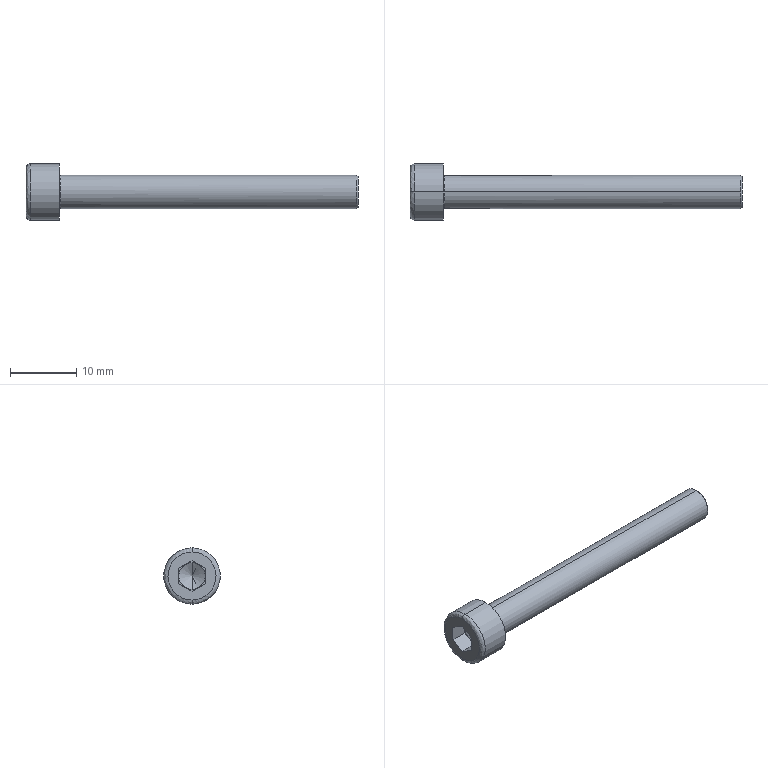Part | SolidWorks | features BaseBody 1 | 1 solid | 27 faces | box 50 x 8.5 x 8.5 mm | volume 1125 mm3 | plane 15 | spline 4 | cylinder 4 | cone 4 | commonest cylinder face diameters 5 x2 8.5 x2
STEP:
#1=CARTESIAN_POINT('',(5.,0.,2.7));
#2=VERTEX_POINT('',#1);
#3=CARTESIAN_POINT('',(5.,0.,-2.7));
#4=VERTEX_POINT('',#3);
#5=CARTESIAN_POINT('',(5.,0.,2.7));
#6=CARTESIAN_POINT('',(5.,0.1716,2.7));
#7=CARTESIAN_POINT('',(5.,0.4245,2.676));
#8=CARTESIAN_POINT('',(5.,0.7118,2.607));
#9=CARTESIAN_POINT('',(5.,0.8535,2.562));
#10=CARTESIAN_POINT('',(5.,0.9138,2.541));
#11=CARTESIAN_POINT('',(5.,0.9539,2.526));
#12=CARTESIAN_POINT('',(5.,0.9722,2.519));
#13=CARTESIAN_POINT('',(5.,1.34,2.373));
#14=CARTESIAN_POINT('',(5.,1.646,2.172));
#15=CARTESIAN_POINT('',(5.,2.041,1.778));
#16=CARTESIAN_POINT('',(5.,2.215,1.564));
#17=CARTESIAN_POINT('',(5.,2.376,1.288));
#18=CARTESIAN_POINT('',(5.,2.447,1.143));
#19=CARTESIAN_POINT('',(5.,2.475,1.08));
#20=CARTESIAN_POINT('',(5.,2.493,1.037));
#21=CARTESIAN_POINT('',(5.,2.503,1.014));
#22=CARTESIAN_POINT('',(5.,2.637,0.675));
#23=CARTESIAN_POINT('',(5.,2.7,0.343));
#24=CARTESIAN_POINT('',(5.,2.7,-0.1715));
#25=CARTESIAN_POINT('',(5.,2.676,-0.4243));
#26=CARTESIAN_POINT('',(5.,2.607,-0.7117));
#27=CARTESIAN_POINT('',(5.,2.562,-0.8534));
#28=CARTESIAN_POINT('',(5.,2.541,-0.9137));
#29=CARTESIAN_POINT('',(5.,2.526,-0.9539));
#30=CARTESIAN_POINT('',(5.,2.519,-0.9722));
#31=CARTESIAN_POINT('',(5.,2.373,-1.34));
#32=CARTESIAN_POINT('',(5.,2.172,-1.646));
#33=CARTESIAN_POINT('',(5.,1.778,-2.041));
#34=CARTESIAN_POINT('',(5.,1.564,-2.215));
#35=CARTESIAN_POINT('',(5.,1.288,-2.376));
#36=CARTESIAN_POINT('',(5.,1.143,-2.447));
#37=CARTESIAN_POINT('',(5.,1.08,-2.475));
#38=CARTESIAN_POINT('',(5.,1.037,-2.493));
#39=CARTESIAN_POINT('',(5.,1.014,-2.503));
#40=CARTESIAN_POINT('',(5.,0.6748,-2.637));
#41=CARTESIAN_POINT('',(5.,0.3435,-2.7));
#42=CARTESIAN_POINT('',(5.,0.,-2.7));
#43=B_SPLINE_CURVE_WITH_KNOTS('',3,(#5,#6,#7,#8,#9,#10,#11,#12,#13,#14,#15,#16,#17,#18,#19,#20,#21,#22,#23,#24,#25,#26,#27,#28,#29,#30,#31,#32,#33,#34,#35,#36,#37,#38,#39,#40,#41,#42),.UNSPECIFIED.,.F.,.F.,(4,1,1,1,2,2,2,1,1,1,2,2,2,1,1,1,2,2,2,1,1,1,2,2,4),(0.,0.0625,0.09375,0.1094,0.1172,0.125,0.25,0.3125,0.3437,0.3594,0.3672,0.375,0.5,0.5625,0.5937,0.6094,0.6172,0.625,0.75,0.8125,0.8437,0.8594,0.8672,0.875,1.),.UNSPECIFIED.);
#44=EDGE_CURVE('',#2,#4,#43,.T.);
#45=ORIENTED_EDGE('',*,*,#44,.F.);
#46=CARTESIAN_POINT('',(5.2,0.,2.5));
#47=VERTEX_POINT('',#46);
#48=CARTESIAN_POINT('',(5.2,0.,2.7));
#49=DIRECTION('',(0.,-1.,0.));
#50=DIRECTION('',(0.,0.,1.));
#51=AXIS2_PLACEMENT_3D('',#48,#49,#50);
#52=CIRCLE('',#51,0.2);
#53=EDGE_CURVE('',#2,#47,#52,.T.);
#54=ORIENTED_EDGE('',*,*,#53,.T.);
#55=CARTESIAN_POINT('',(5.2,0.,-2.5));
#56=VERTEX_POINT('',#55);
#57=CARTESIAN_POINT('',(5.2,0.,0.));
#58=DIRECTION('',(1.,0.,0.));
#59=DIRECTION('',(0.,0.,1.));
#60=AXIS2_PLACEMENT_3D('',#57,#58,#59);
#61=CIRCLE('',#60,2.5);
#62=EDGE_CURVE('',#56,#47,#61,.T.);
#63=ORIENTED_EDGE('',*,*,#62,.F.);
#64=CARTESIAN_POINT('',(5.2,0.,-2.7));
#65=DIRECTION('',(0.,1.,0.));
#66=DIRECTION('',(0.,0.,-1.));
#67=AXIS2_PLACEMENT_3D('',#64,#65,#66);
#68=CIRCLE('',#67,0.2);
#69=EDGE_CURVE('',#4,#56,#68,.T.);
#70=ORIENTED_EDGE('',*,*,#69,.F.);
#71=EDGE_LOOP('',(#45,#54,#63,#70));
#72=FACE_OUTER_BOUND('',#71,.T.);
#73=CARTESIAN_POINT('',(5.,0.,-2.7));
#74=CARTESIAN_POINT('',(5.,5.4,-2.7));
#75=CARTESIAN_POINT('',(5.,5.4,2.7));
#76=CARTESIAN_POINT('',(5.,0.,2.7));
#77=CARTESIAN_POINT('',(5.,0.,-2.583));
#78=CARTESIAN_POINT('',(5.,5.166,-2.583));
#79=CARTESIAN_POINT('',(5.,5.166,2.583));
#80=CARTESIAN_POINT('',(5.,0.,2.583));
#81=CARTESIAN_POINT('',(5.083,0.,-2.5));
#82=CARTESIAN_POINT('',(5.083,5.,-2.5));
#83=CARTESIAN_POINT('',(5.083,5.,2.5));
#84=CARTESIAN_POINT('',(5.083,0.,2.5));
#85=CARTESIAN_POINT('',(5.2,0.,-2.5));
#86=CARTESIAN_POINT('',(5.2,5.,-2.5));
#87=CARTESIAN_POINT('',(5.2,5.,2.5));
#88=CARTESIAN_POINT('',(5.2,0.,2.5));
#89=(BOUNDED_SURFACE()B_SPLINE_SURFACE(3,3,((#73,#74,#75,#76),(#77,#78,#79,#80),(#81,#82,#83,#84),(#85,#86,#87,#88)),.UNSPECIFIED.,.F.,.F.,.F.)B_SPLINE_SURFACE_WITH_KNOTS((4,4),(4,4),(0.,1.),(0.,1.),.UNSPECIFIED.)GEOMETRIC_REPRESENTATION_ITEM()RATIONAL_B_SPLINE_SURFACE(((1.,0.3333,0.3333,1.),(0.8047,0.2682,0.2682,0.8047),(0.8047,0.2682,0.2682,0.8047),(1.,0.3333,0.3333,1.)))REPRESENTATION_ITEM('')SURFACE());
#90=ADVANCED_FACE('',(#72),#89,.F.);
#91=CARTESIAN_POINT('',(0.625,0.,4.25));
#92=VERTEX_POINT('',#91);
#93=CARTESIAN_POINT('',(0.625,0.,-4.25));
#94=VERTEX_POINT('',#93);
#95=CARTESIAN_POINT('',(0.625,0.,0.));
#96=DIRECTION('',(1.,0.,0.));
#97=DIRECTION('',(0.,0.,1.));
#98=AXIS2_PLACEMENT_3D('',#95,#96,#97);
#99=CIRCLE('',#98,4.25);
#100=EDGE_CURVE('',#92,#94,#99,.T.);
#101=ORIENTED_EDGE('',*,*,#100,.F.);
#102=CARTESIAN_POINT('',(0.,0.,3.625));
#103=VERTEX_POINT('',#102);
#104=CARTESIAN_POINT('',(0.625,0.,3.625));
#105=DIRECTION('',(0.,-1.,0.));
#106=DIRECTION('',(0.,0.,1.));
#107=AXIS2_PLACEMENT_3D('',#104,#105,#106);
#108=CIRCLE('',#107,0.625);
#109=EDGE_CURVE('',#92,#103,#108,.T.);
#110=ORIENTED_EDGE('',*,*,#109,.T.);
#111=CARTESIAN_POINT('',(0.,0.,-3.625));
#112=VERTEX_POINT('',#111);
#113=CARTESIAN_POINT('',(0.,0.,3.625));
#114=CARTESIAN_POINT('',(0.,-7.25,3.625));
#115=CARTESIAN_POINT('',(0.,-7.25,-3.625));
#116=CARTESIAN_POINT('',(0.,0.,-3.625));
#117=(BOUNDED_CURVE()B_SPLINE_CURVE(3,(#113,#114,#115,#116),.UNSPECIFIED.,.F.,.F.)B_SPLINE_CURVE_WITH_KNOTS((4,4),(0.,1.),.UNSPECIFIED.)CURVE()GEOMETRIC_REPRESENTATION_ITEM()RATIONAL_B_SPLINE_CURVE((1.,0.3333,0.3333,1.))REPRESENTATION_ITEM(''));
#118=EDGE_CURVE('',#103,#112,#117,.T.);
#119=ORIENTED_EDGE('',*,*,#118,.T.);
#120=CARTESIAN_POINT('',(0.625,0.,-3.625));
#121=DIRECTION('',(0.,1.,0.));
#122=DIRECTION('',(0.,0.,-1.));
#123=AXIS2_PLACEMENT_3D('',#120,#121,#122);
#124=CIRCLE('',#123,0.625);
#125=EDGE_CURVE('',#94,#112,#124,.T.);
#126=ORIENTED_EDGE('',*,*,#125,.F.);
#127=EDGE_LOOP('',(#101,#110,#119,#126));
#128=FACE_OUTER_BOUND('',#127,.T.);
#129=CARTESIAN_POINT('',(0.625,0.,4.25));
#130=CARTESIAN_POINT('',(0.625,-8.5,4.25));
#131=CARTESIAN_POINT('',(0.625,-8.5,-4.25));
#132=CARTESIAN_POINT('',(0.625,0.,-4.25));
#133=CARTESIAN_POINT('',(0.2589,0.,4.25));
#134=CARTESIAN_POINT('',(0.2589,-8.5,4.25));
#135=CARTESIAN_POINT('',(0.2589,-8.5,-4.25));
#136=CARTESIAN_POINT('',(0.2589,0.,-4.25));
#137=CARTESIAN_POINT('',(0.,0.,3.991));
#138=CARTESIAN_POINT('',(0.,-7.982,3.991));
#139=CARTESIAN_POINT('',(0.,-7.982,-3.991));
#140=CARTESIAN_POINT('',(0.,0.,-3.991));
#141=CARTESIAN_POINT('',(0.,0.,3.625));
#142=CARTESIAN_POINT('',(0.,-7.25,3.625));
#143=CARTESIAN_POINT('',(0.,-7.25,-3.625));
#144=CARTESIAN_POINT('',(0.,0.,-3.625));
#145=(BOUNDED_SURFACE()B_SPLINE_SURFACE(3,3,((#129,#130,#131,#132),(#133,#134,#135,#136),(#137,#138,#139,#140),(#141,#142,#143,#144)),.UNSPECIFIED.,.F.,.F.,.T.)B_SPLINE_SURFACE_WITH_KNOTS((4,4),(4,4),(0.,1.),(0.,1.),.UNSPECIFIED.)GEOMETRIC_REPRESENTATION_ITEM()RATIONAL_B_SPLINE_SURFACE(((1.,0.3333,0.3333,1.),(0.8047,0.2682,0.2682,0.8047),(0.8047,0.2682,0.2682,0.8047),(1.,0.3333,0.3333,1.)))REPRESENTATION_ITEM('')SURFACE());
#146=ADVANCED_FACE('',(#128),#145,.T.);
#147=CARTESIAN_POINT('',(49.8,2.5,0.));
#148=VERTEX_POINT('',#147);
#149=CARTESIAN_POINT('',(49.8,0.,-2.5));
#150=VERTEX_POINT('',#149);
#151=CARTESIAN_POINT('',(49.8,0.,0.));
#152=DIRECTION('',(-1.,0.,0.));
#153=DIRECTION('',(0.,0.,1.));
#154=AXIS2_PLACEMENT_3D('',#151,#152,#153);
#155=CIRCLE('',#154,2.5);
#156=EDGE_CURVE('',#148,#150,#155,.T.);
#157=ORIENTED_EDGE('',*,*,#156,.T.);
#158=CARTESIAN_POINT('',(50.,0.,-2.5));
#159=DIRECTION('',(-1.,0.,0.));
#160=VECTOR('',#159,1000.);
#161=LINE('',#158,#160);
#162=EDGE_CURVE('',#150,#56,#161,.T.);
#163=ORIENTED_EDGE('',*,*,#162,.T.);
#164=ORIENTED_EDGE('',*,*,#62,.T.);
#165=CARTESIAN_POINT('',(49.8,0.,2.5));
#166=VERTEX_POINT('',#165);
#167=CARTESIAN_POINT('',(50.,0.,2.5));
#168=DIRECTION('',(-1.,0.,0.));
#169=VECTOR('',#168,1000.);
#170=LINE('',#167,#169);
#171=EDGE_CURVE('',#166,#47,#170,.T.);
#172=ORIENTED_EDGE('',*,*,#171,.F.);
#173=CARTESIAN_POINT('',(49.8,0.,0.));
#174=DIRECTION('',(-1.,0.,0.));
#175=DIRECTION('',(0.,0.,1.));
#176=AXIS2_PLACEMENT_3D('',#173,#174,#175);
#177=CIRCLE('',#176,2.5);
#178=EDGE_CURVE('',#166,#148,#177,.T.);
#179=ORIENTED_EDGE('',*,*,#178,.T.);
#180=EDGE_LOOP('',(#157,#163,#164,#172,#179));
#181=FACE_OUTER_BOUND('',#180,.T.);
#182=CARTESIAN_POINT('',(50.,0.,0.));
#183=DIRECTION('',(-1.,0.,0.));
#184=DIRECTION('',(0.,0.,1.));
#185=AXIS2_PLACEMENT_3D('',#182,#183,#184);
#186=CYLINDRICAL_SURFACE('',#185,2.5);
#187=ADVANCED_FACE('',(#181),#186,.T.);
#188=CARTESIAN_POINT('',(50.,-2.3,0.));
#189=VERTEX_POINT('',#188);
#190=CARTESIAN_POINT('',(50.,2.3,0.));
#191=VERTEX_POINT('',#190);
#192=CARTESIAN_POINT('',(50.,0.,0.));
#193=DIRECTION('',(-1.,0.,0.));
#194=DIRECTION('',(0.,-1.,0.));
#195=AXIS2_PLACEMENT_3D('',#192,#193,#194);
#196=CIRCLE('',#195,2.3);
#197=EDGE_CURVE('',#189,#191,#196,.T.);
#198=ORIENTED_EDGE('',*,*,#197,.T.);
#199=CARTESIAN_POINT('',(49.8,2.5,0.));
#200=DIRECTION('',(-0.7071,0.7071,0.));
#201=VECTOR('',#200,1000.);
#202=LINE('',#199,#201);
#203=EDGE_CURVE('',#191,#148,#202,.T.);
#204=ORIENTED_EDGE('',*,*,#203,.T.);
#205=ORIENTED_EDGE('',*,*,#178,.F.);
#206=CARTESIAN_POINT('',(49.8,-2.5,0.));
#207=VERTEX_POINT('',#206);
#208=CARTESIAN_POINT('',(49.8,0.,0.));
#209=DIRECTION('',(-1.,0.,0.));
#210=DIRECTION('',(0.,0.,1.));
#211=AXIS2_PLACEMENT_3D('',#208,#209,#210);
#212=CIRCLE('',#211,2.5);
#213=EDGE_CURVE('',#207,#166,#212,.T.);
#214=ORIENTED_EDGE('',*,*,#213,.F.);
#215=CARTESIAN_POINT('',(49.8,-2.5,0.));
#216=DIRECTION('',(-0.7071,-0.7071,0.));
#217=VECTOR('',#216,1000.);
#218=LINE('',#215,#217);
#219=EDGE_CURVE('',#189,#207,#218,.T.);
#220=ORIENTED_EDGE('',*,*,#219,.F.);
#221=EDGE_LOOP('',(#198,#204,#205,#214,#220));
#222=FACE_OUTER_BOUND('',#221,.T.);
#223=CARTESIAN_POINT('',(49.8,0.,0.));
#224=DIRECTION('',(-1.,0.,0.));
#225=DIRECTION('',(0.,-1.,0.));
#226=AXIS2_PLACEMENT_3D('',#223,#224,#225);
#227=CONICAL_SURFACE('',#226,2.5,0.7854);
#228=ADVANCED_FACE('',(#222),#227,.T.);
#229=CARTESIAN_POINT('',(5.,0.,-4.25));
#230=VERTEX_POINT('',#229);
#231=CARTESIAN_POINT('',(5.,0.,4.25));
#232=VERTEX_POINT('',#231);
#233=CARTESIAN_POINT('',(5.,0.,0.));
#234=DIRECTION('',(1.,0.,0.));
#235=DIRECTION('',(0.,0.,1.));
#236=AXIS2_PLACEMENT_3D('',#233,#234,#235);
#237=CIRCLE('',#236,4.25);
#238=EDGE_CURVE('',#230,#232,#237,.T.);
#239=ORIENTED_EDGE('',*,*,#238,.F.);
#240=CARTESIAN_POINT('',(5.,0.,-4.25));
#241=DIRECTION('',(-1.,0.,0.));
#242=VECTOR('',#241,1000.);
#243=LINE('',#240,#242);
#244=EDGE_CURVE('',#230,#94,#243,.T.);
#245=ORIENTED_EDGE('',*,*,#244,.T.);
#246=CARTESIAN_POINT('',(0.625,0.,0.));
#247=DIRECTION('',(1.,0.,0.));
#248=DIRECTION('',(0.,0.,1.));
#249=AXIS2_PLACEMENT_3D('',#246,#247,#248);
#250=CIRCLE('',#249,4.25);
#251=EDGE_CURVE('',#94,#92,#250,.T.);
#252=ORIENTED_EDGE('',*,*,#251,.T.);
#253=CARTESIAN_POINT('',(5.,0.,4.25));
#254=DIRECTION('',(-1.,0.,0.));
#255=VECTOR('',#254,1000.);
#256=LINE('',#253,#255);
#257=EDGE_CURVE('',#232,#92,#256,.T.);
#258=ORIENTED_EDGE('',*,*,#257,.F.);
#259=EDGE_LOOP('',(#239,#245,#252,#258));
#260=FACE_OUTER_BOUND('',#259,.T.);
#261=CARTESIAN_POINT('',(5.,0.,0.));
#262=DIRECTION('',(-1.,0.,0.));
#263=DIRECTION('',(0.,0.,1.));
#264=AXIS2_PLACEMENT_3D('',#261,#262,#263);
#265=CYLINDRICAL_SURFACE('',#264,4.25);
#266=ADVANCED_FACE('',(#260),#265,.T.);
#267=CARTESIAN_POINT('',(3.655,0.,0.));
#268=VERTEX_POINT('',#267);
#269=CARTESIAN_POINT('',(2.5,0.,2.));
#270=VERTEX_POINT('',#269);
#271=CARTESIAN_POINT('',(2.5,0.,2.));
#272=DIRECTION('',(-0.5,0.,0.866));
#273=VECTOR('',#272,1000.);
#274=LINE('',#271,#273);
#275=EDGE_CURVE('',#268,#270,#274,.T.);
#276=ORIENTED_EDGE('',*,*,#275,.F.);
#277=CARTESIAN_POINT('',(2.5,0.,-2.));
#278=VERTEX_POINT('',#277);
#279=CARTESIAN_POINT('',(2.5,0.,-2.));
#280=DIRECTION('',(-0.5,0.,-0.866));
#281=VECTOR('',#280,1000.);
#282=LINE('',#279,#281);
#283=EDGE_CURVE('',#268,#278,#282,.T.);
#284=ORIENTED_EDGE('',*,*,#283,.T.);
#285=CARTESIAN_POINT('',(2.5,-1.,-1.732));
#286=VERTEX_POINT('',#285);
#287=CARTESIAN_POINT('',(2.5,0.,0.));
#288=DIRECTION('',(1.,0.,0.));
#289=DIRECTION('',(0.,0.,1.));
#290=AXIS2_PLACEMENT_3D('',#287,#288,#289);
#291=CIRCLE('',#290,2.);
#292=EDGE_CURVE('',#286,#278,#291,.T.);
#293=ORIENTED_EDGE('',*,*,#292,.F.);
#294=CARTESIAN_POINT('',(2.5,-2.,0.));
#295=VERTEX_POINT('',#294);
#296=CARTESIAN_POINT('',(2.5,0.,0.));
#297=DIRECTION('',(-1.,0.,0.));
#298=DIRECTION('',(0.,0.,1.));
#299=AXIS2_PLACEMENT_3D('',#296,#297,#298);
#300=CIRCLE('',#299,2.);
#301=EDGE_CURVE('',#286,#295,#300,.T.);
#302=ORIENTED_EDGE('',*,*,#301,.T.);
#303=CARTESIAN_POINT('',(2.5,-1.,1.732));
#304=VERTEX_POINT('',#303);
#305=CARTESIAN_POINT('',(2.5,0.,0.));
#306=DIRECTION('',(1.,0.,0.));
#307=DIRECTION('',(0.,0.,1.));
#308=AXIS2_PLACEMENT_3D('',#305,#306,#307);
#309=CIRCLE('',#308,2.);
#310=EDGE_CURVE('',#304,#295,#309,.T.);
#311=ORIENTED_EDGE('',*,*,#310,.F.);
#312=CARTESIAN_POINT('',(2.5,0.,0.));
#313=DIRECTION('',(1.,0.,0.));
#314=DIRECTION('',(0.,0.,1.));
#315=AXIS2_PLACEMENT_3D('',#312,#313,#314);
#316=CIRCLE('',#315,2.);
#317=EDGE_CURVE('',#270,#304,#316,.T.);
#318=ORIENTED_EDGE('',*,*,#317,.F.);
#319=EDGE_LOOP('',(#276,#284,#293,#302,#311,#318));
#320=FACE_OUTER_BOUND('',#319,.T.);
#321=CARTESIAN_POINT('',(2.5,0.,0.));
#322=DIRECTION('',(-1.,0.,0.));
#323=DIRECTION('',(0.,0.,1.));
#324=AXIS2_PLACEMENT_3D('',#321,#322,#323);
#325=CONICAL_SURFACE('',#324,2.,1.047);
#326=ADVANCED_FACE('',(#320),#325,.F.);
#327=ORIENTED_EDGE('',*,*,#162,.F.);
#328=CARTESIAN_POINT('',(49.8,0.,0.));
#329=DIRECTION('',(-1.,0.,0.));
#330=DIRECTION('',(0.,0.,1.));
#331=AXIS2_PLACEMENT_3D('',#328,#329,#330);
#332=CIRCLE('',#331,2.5);
#333=EDGE_CURVE('',#150,#207,#332,.T.);
#334=ORIENTED_EDGE('',*,*,#333,.T.);
#335=ORIENTED_EDGE('',*,*,#213,.T.);
#336=ORIENTED_EDGE('',*,*,#171,.T.);
#337=CARTESIAN_POINT('',(5.2,0.,0.));
#338=DIRECTION('',(1.,0.,0.));
#339=DIRECTION('',(0.,0.,1.));
#340=AXIS2_PLACEMENT_3D('',#337,#338,#339);
#341=CIRCLE('',#340,2.5);
#342=EDGE_CURVE('',#47,#56,#341,.T.);
#343=ORIENTED_EDGE('',*,*,#342,.T.);
#344=EDGE_LOOP('',(#327,#334,#335,#336,#343));
#345=FACE_OUTER_BOUND('',#344,.T.);
#346=CARTESIAN_POINT('',(50.,0.,0.));
#347=DIRECTION('',(-1.,0.,0.));
#348=DIRECTION('',(0.,0.,1.));
#349=AXIS2_PLACEMENT_3D('',#346,#347,#348);
#350=CYLINDRICAL_SURFACE('',#349,2.5);
#351=ADVANCED_FACE('',(#345),#350,.T.);
#352=ORIENTED_EDGE('',*,*,#53,.F.);
#353=CARTESIAN_POINT('',(5.,0.,-2.7));
#354=CARTESIAN_POINT('',(5.,-0.1716,-2.7));
#355=CARTESIAN_POINT('',(5.,-0.4245,-2.676));
#356=CARTESIAN_POINT('',(5.,-0.7118,-2.607));
#357=CARTESIAN_POINT('',(5.,-0.8535,-2.562));
#358=CARTESIAN_POINT('',(5.,-0.9138,-2.541));
#359=CARTESIAN_POINT('',(5.,-0.9539,-2.526));
#360=CARTESIAN_POINT('',(5.,-0.9722,-2.519));
#361=CARTESIAN_POINT('',(5.,-1.34,-2.373));
#362=CARTESIAN_POINT('',(5.,-1.646,-2.172));
#363=CARTESIAN_POINT('',(5.,-2.041,-1.778));
#364=CARTESIAN_POINT('',(5.,-2.215,-1.564));
#365=CARTESIAN_POINT('',(5.,-2.376,-1.288));
#366=CARTESIAN_POINT('',(5.,-2.447,-1.143));
#367=CARTESIAN_POINT('',(5.,-2.475,-1.08));
#368=CARTESIAN_POINT('',(5.,-2.493,-1.037));
#369=CARTESIAN_POINT('',(5.,-2.503,-1.014));
#370=CARTESIAN_POINT('',(5.,-2.637,-0.675));
#371=CARTESIAN_POINT('',(5.,-2.7,-0.343));
#372=CARTESIAN_POINT('',(5.,-2.7,0.1715));
#373=CARTESIAN_POINT('',(5.,-2.676,0.4243));
#374=CARTESIAN_POINT('',(5.,-2.607,0.7117));
#375=CARTESIAN_POINT('',(5.,-2.562,0.8534));
#376=CARTESIAN_POINT('',(5.,-2.541,0.9137));
#377=CARTESIAN_POINT('',(5.,-2.526,0.9539));
#378=CARTESIAN_POINT('',(5.,-2.519,0.9722));
#379=CARTESIAN_POINT('',(5.,-2.373,1.34));
#380=CARTESIAN_POINT('',(5.,-2.172,1.646));
#381=CARTESIAN_POINT('',(5.,-1.778,2.041));
#382=CARTESIAN_POINT('',(5.,-1.564,2.215));
#383=CARTESIAN_POINT('',(5.,-1.288,2.376));
#384=CARTESIAN_POINT('',(5.,-1.143,2.447));
#385=CARTESIAN_POINT('',(5.,-1.08,2.475));
#386=CARTESIAN_POINT('',(5.,-1.037,2.493));
#387=CARTESIAN_POINT('',(5.,-1.014,2.503));
#388=CARTESIAN_POINT('',(5.,-0.6748,2.637));
#389=CARTESIAN_POINT('',(5.,-0.3435,2.7));
#390=CARTESIAN_POINT('',(5.,0.,2.7));
#391=B_SPLINE_CURVE_WITH_KNOTS('',3,(#353,#354,#355,#356,#357,#358,#359,#360,#361,#362,#363,#364,#365,#366,#367,#368,#369,#370,#371,#372,#373,#374,#375,#376,#377,#378,#379,#380,#381,#382,#383,#384,#385,#386,#387,#388,#389,#390),.UNSPECIFIED.,.F.,.F.,(4,1,1,1,2,2,2,1,1,1,2,2,2,1,1,1,2,2,2,1,1,1,2,2,4),(0.,0.0625,0.09375,0.1094,0.1172,0.125,0.25,0.3125,0.3437,0.3594,0.3672,0.375,0.5,0.5625,0.5937,0.6094,0.6172,0.625,0.75,0.8125,0.8437,0.8594,0.8672,0.875,1.),.UNSPECIFIED.);
#392=EDGE_CURVE('',#4,#2,#391,.T.);
#393=ORIENTED_EDGE('',*,*,#392,.F.);
#394=ORIENTED_EDGE('',*,*,#69,.T.);
#395=ORIENTED_EDGE('',*,*,#342,.F.);
#396=EDGE_LOOP('',(#352,#393,#394,#395));
#397=FACE_OUTER_BOUND('',#396,.T.);
#398=CARTESIAN_POINT('',(5.,0.,2.7));
#399=CARTESIAN_POINT('',(5.,-5.4,2.7));
#400=CARTESIAN_POINT('',(5.,-5.4,-2.7));
#401=CARTESIAN_POINT('',(5.,0.,-2.7));
#402=CARTESIAN_POINT('',(5.,0.,2.583));
#403=CARTESIAN_POINT('',(5.,-5.166,2.583));
#404=CARTESIAN_POINT('',(5.,-5.166,-2.583));
#405=CARTESIAN_POINT('',(5.,0.,-2.583));
#406=CARTESIAN_POINT('',(5.083,0.,2.5));
#407=CARTESIAN_POINT('',(5.083,-5.,2.5));
#408=CARTESIAN_POINT('',(5.083,-5.,-2.5));
#409=CARTESIAN_POINT('',(5.083,0.,-2.5));
#410=CARTESIAN_POINT('',(5.2,0.,2.5));
#411=CARTESIAN_POINT('',(5.2,-5.,2.5));
#412=CARTESIAN_POINT('',(5.2,-5.,-2.5));
#413=CARTESIAN_POINT('',(5.2,0.,-2.5));
#414=(BOUNDED_SURFACE()B_SPLINE_SURFACE(3,3,((#398,#399,#400,#401),(#402,#403,#404,#405),(#406,#407,#408,#409),(#410,#411,#412,#413)),.UNSPECIFIED.,.F.,.F.,.T.)B_SPLINE_SURFACE_WITH_KNOTS((4,4),(4,4),(0.,1.),(0.,1.),.UNSPECIFIED.)GEOMETRIC_REPRESENTATION_ITEM()RATIONAL_B_SPLINE_SURFACE(((1.,0.3333,0.3333,1.),(0.8047,0.2682,0.2682,0.8047),(0.8047,0.2682,0.2682,0.8047),(1.,0.3333,0.3333,1.)))REPRESENTATION_ITEM('')SURFACE());
#415=ADVANCED_FACE('',(#397),#414,.F.);
#416=ORIENTED_EDGE('',*,*,#203,.F.);
#417=CARTESIAN_POINT('',(50.,0.,0.));
#418=DIRECTION('',(-1.,0.,0.));
#419=DIRECTION('',(0.,-1.,0.));
#420=AXIS2_PLACEMENT_3D('',#417,#418,#419);
#421=CIRCLE('',#420,2.3);
#422=EDGE_CURVE('',#191,#189,#421,.T.);
#423=ORIENTED_EDGE('',*,*,#422,.T.);
#424=ORIENTED_EDGE('',*,*,#219,.T.);
#425=ORIENTED_EDGE('',*,*,#333,.F.);
#426=ORIENTED_EDGE('',*,*,#156,.F.);
#427=EDGE_LOOP('',(#416,#423,#424,#425,#426));
#428=FACE_OUTER_BOUND('',#427,.T.);
#429=CARTESIAN_POINT('',(49.8,0.,0.));
#430=DIRECTION('',(-1.,0.,0.));
#431=DIRECTION('',(0.,-1.,0.));
#432=AXIS2_PLACEMENT_3D('',#429,#430,#431);
#433=CONICAL_SURFACE('',#432,2.5,0.7854);
#434=ADVANCED_FACE('',(#428),#433,.T.);
#435=CARTESIAN_POINT('',(5.,0.,0.));
#436=DIRECTION('',(1.,0.,0.));
#437=DIRECTION('',(0.,0.,1.));
#438=AXIS2_PLACEMENT_3D('',#435,#436,#437);
#439=CIRCLE('',#438,4.25);
#440=EDGE_CURVE('',#232,#230,#439,.T.);
#441=ORIENTED_EDGE('',*,*,#440,.T.);
#442=ORIENTED_EDGE('',*,*,#238,.T.);
#443=EDGE_LOOP('',(#441,#442));
#444=FACE_OUTER_BOUND('',#443,.T.);
#445=ORIENTED_EDGE('',*,*,#392,.T.);
#446=ORIENTED_EDGE('',*,*,#44,.T.);
#447=EDGE_LOOP('',(#445,#446));
#448=FACE_BOUND('',#447,.T.);
#449=CARTESIAN_POINT('',(5.,0.,0.));
#450=DIRECTION('',(1.,0.,0.));
#451=DIRECTION('',(0.,0.,-1.));
#452=AXIS2_PLACEMENT_3D('',#449,#450,#451);
#453=PLANE('',#452);
#454=ADVANCED_FACE('',(#444,#448),#453,.T.);
#455=ORIENTED_EDGE('',*,*,#197,.F.);
#456=ORIENTED_EDGE('',*,*,#422,.F.);
#457=EDGE_LOOP('',(#455,#456));
#458=FACE_OUTER_BOUND('',#457,.T.);
#459=CARTESIAN_POINT('',(50.,0.,0.));
#460=DIRECTION('',(1.,0.,0.));
#461=DIRECTION('',(0.,0.,-1.));
#462=AXIS2_PLACEMENT_3D('',#459,#460,#461);
#463=PLANE('',#462);
#464=ADVANCED_FACE('',(#458),#463,.T.);
#465=ORIENTED_EDGE('',*,*,#244,.F.);
#466=ORIENTED_EDGE('',*,*,#440,.F.);
#467=ORIENTED_EDGE('',*,*,#257,.T.);
#468=ORIENTED_EDGE('',*,*,#100,.T.);
#469=EDGE_LOOP('',(#465,#466,#467,#468));
#470=FACE_OUTER_BOUND('',#469,.T.);
#471=CARTESIAN_POINT('',(5.,0.,0.));
#472=DIRECTION('',(-1.,0.,0.));
#473=DIRECTION('',(0.,0.,1.));
#474=AXIS2_PLACEMENT_3D('',#471,#472,#473);
#475=CYLINDRICAL_SURFACE('',#474,4.25);
#476=ADVANCED_FACE('',(#470),#475,.T.);
#477=ORIENTED_EDGE('',*,*,#109,.F.);
#478=ORIENTED_EDGE('',*,*,#251,.F.);
#479=ORIENTED_EDGE('',*,*,#125,.T.);
#480=CARTESIAN_POINT('',(0.,0.,-3.625));
#481=CARTESIAN_POINT('',(0.,7.25,-3.625));
#482=CARTESIAN_POINT('',(0.,7.25,3.625));
#483=CARTESIAN_POINT('',(0.,0.,3.625));
#484=(BOUNDED_CURVE()B_SPLINE_CURVE(3,(#480,#481,#482,#483),.UNSPECIFIED.,.F.,.T.)B_SPLINE_CURVE_WITH_KNOTS((4,4),(0.,1.),.UNSPECIFIED.)CURVE()GEOMETRIC_REPRESENTATION_ITEM()RATIONAL_B_SPLINE_CURVE((1.,0.3333,0.3333,1.))REPRESENTATION_ITEM(''));
#485=EDGE_CURVE('',#112,#103,#484,.T.);
#486=ORIENTED_EDGE('',*,*,#485,.T.);
#487=EDGE_LOOP('',(#477,#478,#479,#486));
#488=FACE_OUTER_BOUND('',#487,.T.);
#489=CARTESIAN_POINT('',(0.625,0.,-4.25));
#490=CARTESIAN_POINT('',(0.625,8.5,-4.25));
#491=CARTESIAN_POINT('',(0.625,8.5,4.25));
#492=CARTESIAN_POINT('',(0.625,0.,4.25));
#493=CARTESIAN_POINT('',(0.2589,0.,-4.25));
#494=CARTESIAN_POINT('',(0.2589,8.5,-4.25));
#495=CARTESIAN_POINT('',(0.2589,8.5,4.25));
#496=CARTESIAN_POINT('',(0.2589,0.,4.25));
#497=CARTESIAN_POINT('',(0.,0.,-3.991));
#498=CARTESIAN_POINT('',(0.,7.982,-3.991));
#499=CARTESIAN_POINT('',(0.,7.982,3.991));
#500=CARTESIAN_POINT('',(0.,0.,3.991));
#501=CARTESIAN_POINT('',(0.,0.,-3.625));
#502=CARTESIAN_POINT('',(0.,7.25,-3.625));
#503=CARTESIAN_POINT('',(0.,7.25,3.625));
#504=CARTESIAN_POINT('',(0.,0.,3.625));
#505=(BOUNDED_SURFACE()B_SPLINE_SURFACE(3,3,((#489,#490,#491,#492),(#493,#494,#495,#496),(#497,#498,#499,#500),(#501,#502,#503,#504)),.UNSPECIFIED.,.F.,.F.,.F.)B_SPLINE_SURFACE_WITH_KNOTS((4,4),(4,4),(0.,1.),(0.,1.),.UNSPECIFIED.)GEOMETRIC_REPRESENTATION_ITEM()RATIONAL_B_SPLINE_SURFACE(((1.,0.3333,0.3333,1.),(0.8047,0.2682,0.2682,0.8047),(0.8047,0.2682,0.2682,0.8047),(1.,0.3333,0.3333,1.)))REPRESENTATION_ITEM('')SURFACE());
#506=ADVANCED_FACE('',(#488),#505,.T.);
#507=CARTESIAN_POINT('',(0.,2.,1.155));
#508=VERTEX_POINT('',#507);
#509=CARTESIAN_POINT('',(0.,2.,-1.155));
#510=VERTEX_POINT('',#509);
#511=CARTESIAN_POINT('',(0.,2.,0.));
#512=DIRECTION('',(0.,0.,-1.));
#513=VECTOR('',#512,1000.);
#514=LINE('',#511,#513);
#515=EDGE_CURVE('',#508,#510,#514,.T.);
#516=ORIENTED_EDGE('',*,*,#515,.F.);
#517=CARTESIAN_POINT('',(0.,0.,2.309));
#518=VERTEX_POINT('',#517);
#519=CARTESIAN_POINT('',(0.,0.,2.309));
#520=DIRECTION('',(0.,0.866,-0.5));
#521=VECTOR('',#520,1000.);
#522=LINE('',#519,#521);
#523=EDGE_CURVE('',#518,#508,#522,.T.);
#524=ORIENTED_EDGE('',*,*,#523,.F.);
#525=CARTESIAN_POINT('',(0.,-2.,1.155));
#526=VERTEX_POINT('',#525);
#527=CARTESIAN_POINT('',(0.,-2.,1.155));
#528=DIRECTION('',(0.,0.866,0.5));
#529=VECTOR('',#528,1000.);
#530=LINE('',#527,#529);
#531=EDGE_CURVE('',#526,#518,#530,.T.);
#532=ORIENTED_EDGE('',*,*,#531,.F.);
#533=CARTESIAN_POINT('',(0.,-2.,-1.155));
#534=VERTEX_POINT('',#533);
#535=CARTESIAN_POINT('',(0.,-2.,0.));
#536=DIRECTION('',(0.,0.,1.));
#537=VECTOR('',#536,1000.);
#538=LINE('',#535,#537);
#539=EDGE_CURVE('',#534,#526,#538,.T.);
#540=ORIENTED_EDGE('',*,*,#539,.F.);
#541=CARTESIAN_POINT('',(0.,0.,-2.309));
#542=VERTEX_POINT('',#541);
#543=CARTESIAN_POINT('',(0.,0.,-2.309));
#544=DIRECTION('',(0.,-0.866,0.5));
#545=VECTOR('',#544,1000.);
#546=LINE('',#543,#545);
#547=EDGE_CURVE('',#542,#534,#546,.T.);
#548=ORIENTED_EDGE('',*,*,#547,.F.);
#549=CARTESIAN_POINT('',(0.,2.,-1.155));
#550=DIRECTION('',(0.,-0.866,-0.5));
#551=VECTOR('',#550,1000.);
#552=LINE('',#549,#551);
#553=EDGE_CURVE('',#510,#542,#552,.T.);
#554=ORIENTED_EDGE('',*,*,#553,.F.);
#555=EDGE_LOOP('',(#516,#524,#532,#540,#548,#554));
#556=FACE_BOUND('',#555,.T.);
#557=ORIENTED_EDGE('',*,*,#485,.F.);
#558=ORIENTED_EDGE('',*,*,#118,.F.);
#559=EDGE_LOOP('',(#557,#558));
#560=FACE_OUTER_BOUND('',#559,.T.);
#561=CARTESIAN_POINT('',(0.,0.,0.));
#562=DIRECTION('',(1.,0.,0.));
#563=DIRECTION('',(0.,0.,-1.));
#564=AXIS2_PLACEMENT_3D('',#561,#562,#563);
#565=PLANE('',#564);
#566=ADVANCED_FACE('',(#556,#560),#565,.F.);
#567=CARTESIAN_POINT('',(2.5,0.,-2.309));
#568=VERTEX_POINT('',#567);
#569=CARTESIAN_POINT('',(2.5,0.,-2.309));
#570=DIRECTION('',(1.,0.,0.));
#571=VECTOR('',#570,1000.);
#572=LINE('',#569,#571);
#573=EDGE_CURVE('',#542,#568,#572,.T.);
#574=ORIENTED_EDGE('',*,*,#573,.T.);
#575=CARTESIAN_POINT('',(2.5,1.,-1.732));
#576=VERTEX_POINT('',#575);
#577=CARTESIAN_POINT('',(2.5,0.,-2.309));
#578=DIRECTION('',(0.,0.866,0.5));
#579=VECTOR('',#578,1000.);
#580=LINE('',#577,#579);
#581=EDGE_CURVE('',#568,#576,#580,.T.);
#582=ORIENTED_EDGE('',*,*,#581,.T.);
#583=CARTESIAN_POINT('',(2.5,2.,-1.155));
#584=VERTEX_POINT('',#583);
#585=CARTESIAN_POINT('',(2.5,1.,-1.732));
#586=DIRECTION('',(0.,0.866,0.5));
#587=VECTOR('',#586,1000.);
#588=LINE('',#585,#587);
#589=EDGE_CURVE('',#576,#584,#588,.T.);
#590=ORIENTED_EDGE('',*,*,#589,.T.);
#591=CARTESIAN_POINT('',(2.5,2.,-1.155));
#592=DIRECTION('',(-1.,0.,0.));
#593=VECTOR('',#592,1000.);
#594=LINE('',#591,#593);
#595=EDGE_CURVE('',#584,#510,#594,.T.);
#596=ORIENTED_EDGE('',*,*,#595,.T.);
#597=ORIENTED_EDGE('',*,*,#553,.T.);
#598=EDGE_LOOP('',(#574,#582,#590,#596,#597));
#599=FACE_OUTER_BOUND('',#598,.T.);
#600=CARTESIAN_POINT('',(2.5,0.,-2.309));
#601=DIRECTION('',(0.,-0.5,0.866));
#602=DIRECTION('',(0.,-0.866,-0.5));
#603=AXIS2_PLACEMENT_3D('',#600,#601,#602);
#604=PLANE('',#603);
#605=ADVANCED_FACE('',(#599),#604,.T.);
#606=ORIENTED_EDGE('',*,*,#595,.F.);
#607=CARTESIAN_POINT('',(2.5,2.,0.));
#608=VERTEX_POINT('',#607);
#609=CARTESIAN_POINT('',(2.5,2.,-2.309));
#610=DIRECTION('',(0.,0.,1.));
#611=VECTOR('',#610,1000.);
#612=LINE('',#609,#611);
#613=EDGE_CURVE('',#584,#608,#612,.T.);
#614=ORIENTED_EDGE('',*,*,#613,.T.);
#615=CARTESIAN_POINT('',(2.5,2.,1.155));
#616=VERTEX_POINT('',#615);
#617=CARTESIAN_POINT('',(2.5,2.,-2.309));
#618=DIRECTION('',(0.,0.,1.));
#619=VECTOR('',#618,1000.);
#620=LINE('',#617,#619);
#621=EDGE_CURVE('',#608,#616,#620,.T.);
#622=ORIENTED_EDGE('',*,*,#621,.T.);
#623=CARTESIAN_POINT('',(2.5,2.,1.155));
#624=DIRECTION('',(-1.,0.,0.));
#625=VECTOR('',#624,1000.);
#626=LINE('',#623,#625);
#627=EDGE_CURVE('',#616,#508,#626,.T.);
#628=ORIENTED_EDGE('',*,*,#627,.T.);
#629=ORIENTED_EDGE('',*,*,#515,.T.);
#630=EDGE_LOOP('',(#606,#614,#622,#628,#629));
#631=FACE_OUTER_BOUND('',#630,.T.);
#632=CARTESIAN_POINT('',(2.5,2.,-1.155));
#633=DIRECTION('',(0.,-1.,0.));
#634=DIRECTION('',(0.,0.,-1.));
#635=AXIS2_PLACEMENT_3D('',#632,#633,#634);
#636=PLANE('',#635);
#637=ADVANCED_FACE('',(#631),#636,.T.);
#638=ORIENTED_EDGE('',*,*,#627,.F.);
#639=CARTESIAN_POINT('',(2.5,1.,1.732));
#640=VERTEX_POINT('',#639);
#641=CARTESIAN_POINT('',(2.5,2.,1.155));
#642=DIRECTION('',(0.,-0.866,0.5));
#643=VECTOR('',#642,1000.);
#644=LINE('',#641,#643);
#645=EDGE_CURVE('',#616,#640,#644,.T.);
#646=ORIENTED_EDGE('',*,*,#645,.T.);
#647=CARTESIAN_POINT('',(2.5,0.,2.309));
#648=VERTEX_POINT('',#647);
#649=CARTESIAN_POINT('',(2.5,2.,1.155));
#650=DIRECTION('',(0.,-0.866,0.5));
#651=VECTOR('',#650,1000.);
#652=LINE('',#649,#651);
#653=EDGE_CURVE('',#640,#648,#652,.T.);
#654=ORIENTED_EDGE('',*,*,#653,.T.);
#655=CARTESIAN_POINT('',(2.5,0.,2.309));
#656=DIRECTION('',(-1.,0.,0.));
#657=VECTOR('',#656,1000.);
#658=LINE('',#655,#657);
#659=EDGE_CURVE('',#648,#518,#658,.T.);
#660=ORIENTED_EDGE('',*,*,#659,.T.);
#661=ORIENTED_EDGE('',*,*,#523,.T.);
#662=EDGE_LOOP('',(#638,#646,#654,#660,#661));
#663=FACE_OUTER_BOUND('',#662,.T.);
#664=CARTESIAN_POINT('',(2.5,2.,1.155));
#665=DIRECTION('',(0.,-0.5,-0.866));
#666=DIRECTION('',(0.,0.866,-0.5));
#667=AXIS2_PLACEMENT_3D('',#664,#665,#666);
#668=PLANE('',#667);
#669=ADVANCED_FACE('',(#663),#668,.T.);
#670=ORIENTED_EDGE('',*,*,#659,.F.);
#671=CARTESIAN_POINT('',(2.5,0.,2.309));
#672=DIRECTION('',(0.,-0.866,-0.5));
#673=VECTOR('',#672,1000.);
#674=LINE('',#671,#673);
#675=EDGE_CURVE('',#648,#304,#674,.T.);
#676=ORIENTED_EDGE('',*,*,#675,.T.);
#677=CARTESIAN_POINT('',(2.5,-2.,1.155));
#678=VERTEX_POINT('',#677);
#679=CARTESIAN_POINT('',(2.5,-1.,1.732));
#680=DIRECTION('',(0.,-0.866,-0.5));
#681=VECTOR('',#680,1000.);
#682=LINE('',#679,#681);
#683=EDGE_CURVE('',#304,#678,#682,.T.);
#684=ORIENTED_EDGE('',*,*,#683,.T.);
#685=CARTESIAN_POINT('',(2.5,-2.,1.155));
#686=DIRECTION('',(-1.,0.,0.));
#687=VECTOR('',#686,1000.);
#688=LINE('',#685,#687);
#689=EDGE_CURVE('',#678,#526,#688,.T.);
#690=ORIENTED_EDGE('',*,*,#689,.T.);
#691=ORIENTED_EDGE('',*,*,#531,.T.);
#692=EDGE_LOOP('',(#670,#676,#684,#690,#691));
#693=FACE_OUTER_BOUND('',#692,.T.);
#694=CARTESIAN_POINT('',(2.5,0.,2.309));
#695=DIRECTION('',(0.,0.5,-0.866));
#696=DIRECTION('',(0.,0.866,0.5));
#697=AXIS2_PLACEMENT_3D('',#694,#695,#696);
#698=PLANE('',#697);
#699=ADVANCED_FACE('',(#693),#698,.T.);
#700=ORIENTED_EDGE('',*,*,#689,.F.);
#701=CARTESIAN_POINT('',(2.5,-2.,-2.309));
#702=DIRECTION('',(0.,0.,-1.));
#703=VECTOR('',#702,1000.);
#704=LINE('',#701,#703);
#705=EDGE_CURVE('',#678,#295,#704,.T.);
#706=ORIENTED_EDGE('',*,*,#705,.T.);
#707=CARTESIAN_POINT('',(2.5,-2.,-1.155));
#708=VERTEX_POINT('',#707);
#709=CARTESIAN_POINT('',(2.5,-2.,1.155));
#710=DIRECTION('',(0.,0.,-1.));
#711=VECTOR('',#710,1000.);
#712=LINE('',#709,#711);
#713=EDGE_CURVE('',#295,#708,#712,.T.);
#714=ORIENTED_EDGE('',*,*,#713,.T.);
#715=CARTESIAN_POINT('',(2.5,-2.,-1.155));
#716=DIRECTION('',(-1.,0.,0.));
#717=VECTOR('',#716,1000.);
#718=LINE('',#715,#717);
#719=EDGE_CURVE('',#708,#534,#718,.T.);
#720=ORIENTED_EDGE('',*,*,#719,.T.);
#721=ORIENTED_EDGE('',*,*,#539,.T.);
#722=EDGE_LOOP('',(#700,#706,#714,#720,#721));
#723=FACE_OUTER_BOUND('',#722,.T.);
#724=CARTESIAN_POINT('',(2.5,-2.,1.155));
#725=DIRECTION('',(0.,1.,0.));
#726=DIRECTION('',(0.,0.,1.));
#727=AXIS2_PLACEMENT_3D('',#724,#725,#726);
#728=PLANE('',#727);
#729=ADVANCED_FACE('',(#723),#728,.T.);
#730=ORIENTED_EDGE('',*,*,#719,.F.);
#731=CARTESIAN_POINT('',(2.5,-2.,-1.155));
#732=DIRECTION('',(0.,0.866,-0.5));
#733=VECTOR('',#732,1000.);
#734=LINE('',#731,#733);
#735=EDGE_CURVE('',#708,#286,#734,.T.);
#736=ORIENTED_EDGE('',*,*,#735,.T.);
#737=CARTESIAN_POINT('',(2.5,-2.,-1.155));
#738=DIRECTION('',(0.,0.866,-0.5));
#739=VECTOR('',#738,1000.);
#740=LINE('',#737,#739);
#741=EDGE_CURVE('',#286,#568,#740,.T.);
#742=ORIENTED_EDGE('',*,*,#741,.T.);
#743=ORIENTED_EDGE('',*,*,#573,.F.);
#744=ORIENTED_EDGE('',*,*,#547,.T.);
#745=EDGE_LOOP('',(#730,#736,#742,#743,#744));
#746=FACE_OUTER_BOUND('',#745,.T.);
#747=CARTESIAN_POINT('',(2.5,-2.,-1.155));
#748=DIRECTION('',(0.,0.5,0.866));
#749=DIRECTION('',(0.,-0.866,0.5));
#750=AXIS2_PLACEMENT_3D('',#747,#748,#749);
#751=PLANE('',#750);
#752=ADVANCED_FACE('',(#746),#751,.T.);
#753=ORIENTED_EDGE('',*,*,#292,.T.);
#754=CARTESIAN_POINT('',(2.5,0.,0.));
#755=DIRECTION('',(1.,0.,0.));
#756=DIRECTION('',(0.,0.,1.));
#757=AXIS2_PLACEMENT_3D('',#754,#755,#756);
#758=CIRCLE('',#757,2.);
#759=EDGE_CURVE('',#278,#576,#758,.T.);
#760=ORIENTED_EDGE('',*,*,#759,.T.);
#761=ORIENTED_EDGE('',*,*,#581,.F.);
#762=ORIENTED_EDGE('',*,*,#741,.F.);
#763=EDGE_LOOP('',(#753,#760,#761,#762));
#764=FACE_OUTER_BOUND('',#763,.T.);
#765=CARTESIAN_POINT('',(2.5,0.,-2.309));
#766=DIRECTION('',(1.,0.,0.));
#767=DIRECTION('',(0.,0.,-1.));
#768=AXIS2_PLACEMENT_3D('',#765,#766,#767);
#769=PLANE('',#768);
#770=ADVANCED_FACE('',(#764),#769,.F.);
#771=ORIENTED_EDGE('',*,*,#653,.F.);
#772=CARTESIAN_POINT('',(2.5,0.,0.));
#773=DIRECTION('',(1.,0.,0.));
#774=DIRECTION('',(0.,0.,1.));
#775=AXIS2_PLACEMENT_3D('',#772,#773,#774);
#776=CIRCLE('',#775,2.);
#777=EDGE_CURVE('',#640,#270,#776,.T.);
#778=ORIENTED_EDGE('',*,*,#777,.T.);
#779=ORIENTED_EDGE('',*,*,#317,.T.);
#780=ORIENTED_EDGE('',*,*,#675,.F.);
#781=EDGE_LOOP('',(#771,#778,#779,#780));
#782=FACE_OUTER_BOUND('',#781,.T.);
#783=CARTESIAN_POINT('',(2.5,0.,-2.309));
#784=DIRECTION('',(1.,0.,0.));
#785=DIRECTION('',(0.,0.,-1.));
#786=AXIS2_PLACEMENT_3D('',#783,#784,#785);
#787=PLANE('',#786);
#788=ADVANCED_FACE('',(#782),#787,.F.);
#789=ORIENTED_EDGE('',*,*,#735,.F.);
#790=ORIENTED_EDGE('',*,*,#713,.F.);
#791=ORIENTED_EDGE('',*,*,#301,.F.);
#792=EDGE_LOOP('',(#789,#790,#791));
#793=FACE_OUTER_BOUND('',#792,.T.);
#794=CARTESIAN_POINT('',(2.5,0.,-2.309));
#795=DIRECTION('',(1.,0.,0.));
#796=DIRECTION('',(0.,0.,-1.));
#797=AXIS2_PLACEMENT_3D('',#794,#795,#796);
#798=PLANE('',#797);
#799=ADVANCED_FACE('',(#793),#798,.F.);
#800=ORIENTED_EDGE('',*,*,#283,.F.);
#801=ORIENTED_EDGE('',*,*,#275,.T.);
#802=ORIENTED_EDGE('',*,*,#777,.F.);
#803=CARTESIAN_POINT('',(2.5,0.,0.));
#804=DIRECTION('',(1.,0.,0.));
#805=DIRECTION('',(0.,0.,1.));
#806=AXIS2_PLACEMENT_3D('',#803,#804,#805);
#807=CIRCLE('',#806,2.);
#808=EDGE_CURVE('',#608,#640,#807,.T.);
#809=ORIENTED_EDGE('',*,*,#808,.F.);
#810=CARTESIAN_POINT('',(2.5,0.,0.));
#811=DIRECTION('',(1.,0.,0.));
#812=DIRECTION('',(0.,0.,1.));
#813=AXIS2_PLACEMENT_3D('',#810,#811,#812);
#814=CIRCLE('',#813,2.);
#815=EDGE_CURVE('',#576,#608,#814,.T.);
#816=ORIENTED_EDGE('',*,*,#815,.F.);
#817=ORIENTED_EDGE('',*,*,#759,.F.);
#818=EDGE_LOOP('',(#800,#801,#802,#809,#816,#817));
#819=FACE_OUTER_BOUND('',#818,.T.);
#820=CARTESIAN_POINT('',(2.5,0.,0.));
#821=DIRECTION('',(-1.,0.,0.));
#822=DIRECTION('',(0.,0.,1.));
#823=AXIS2_PLACEMENT_3D('',#820,#821,#822);
#824=CONICAL_SURFACE('',#823,2.,1.047);
#825=ADVANCED_FACE('',(#819),#824,.F.);
#826=ORIENTED_EDGE('',*,*,#705,.F.);
#827=ORIENTED_EDGE('',*,*,#683,.F.);
#828=ORIENTED_EDGE('',*,*,#310,.T.);
#829=EDGE_LOOP('',(#826,#827,#828));
#830=FACE_OUTER_BOUND('',#829,.T.);
#831=CARTESIAN_POINT('',(2.5,0.,-2.309));
#832=DIRECTION('',(1.,0.,0.));
#833=DIRECTION('',(0.,0.,-1.));
#834=AXIS2_PLACEMENT_3D('',#831,#832,#833);
#835=PLANE('',#834);
#836=ADVANCED_FACE('',(#830),#835,.F.);
#837=ORIENTED_EDGE('',*,*,#645,.F.);
#838=ORIENTED_EDGE('',*,*,#621,.F.);
#839=ORIENTED_EDGE('',*,*,#808,.T.);
#840=EDGE_LOOP('',(#837,#838,#839));
#841=FACE_OUTER_BOUND('',#840,.T.);
#842=CARTESIAN_POINT('',(2.5,0.,-2.309));
#843=DIRECTION('',(1.,0.,0.));
#844=DIRECTION('',(0.,0.,-1.));
#845=AXIS2_PLACEMENT_3D('',#842,#843,#844);
#846=PLANE('',#845);
#847=ADVANCED_FACE('',(#841),#846,.F.);
#848=ORIENTED_EDGE('',*,*,#613,.F.);
#849=ORIENTED_EDGE('',*,*,#589,.F.);
#850=ORIENTED_EDGE('',*,*,#815,.T.);
#851=EDGE_LOOP('',(#848,#849,#850));
#852=FACE_OUTER_BOUND('',#851,.T.);
#853=CARTESIAN_POINT('',(2.5,0.,-2.309));
#854=DIRECTION('',(1.,0.,0.));
#855=DIRECTION('',(0.,0.,-1.));
#856=AXIS2_PLACEMENT_3D('',#853,#854,#855);
#857=PLANE('',#856);
#858=ADVANCED_FACE('',(#852),#857,.F.);
#859=CLOSED_SHELL('',(#90,#146,#187,#228,#266,#326,#351,#415,#434,#454,#464,#476,#506,#566,#605,#637,#669,#699,#729,#752,#770,#788,#799,#825,#836,#847,#858));
#860=MANIFOLD_SOLID_BREP('',#859);
#861=CARTESIAN_POINT('',(0.,0.,0.));
#862=DIRECTION('',(0.,0.,1.));
#863=DIRECTION('',(1.,0.,0.));
#864=AXIS2_PLACEMENT_3D('',#861,#862,#863);
#865=(LENGTH_UNIT()NAMED_UNIT(*)SI_UNIT(.MILLI.,.METRE.));
#866=UNCERTAINTY_MEASURE_WITH_UNIT(LENGTH_MEASURE(0.00001),#865,'','');
#867=(NAMED_UNIT(*)PLANE_ANGLE_UNIT()SI_UNIT($,.RADIAN.));
#868=(NAMED_UNIT(*)SI_UNIT($,.STERADIAN.)SOLID_ANGLE_UNIT());
#869=(GEOMETRIC_REPRESENTATION_CONTEXT(3)GLOBAL_UNCERTAINTY_ASSIGNED_CONTEXT((#866))GLOBAL_UNIT_ASSIGNED_CONTEXT((#865,#867,#868))REPRESENTATION_CONTEXT('',''));
#870=ADVANCED_BREP_SHAPE_REPRESENTATION('',(#860,#864),#869);